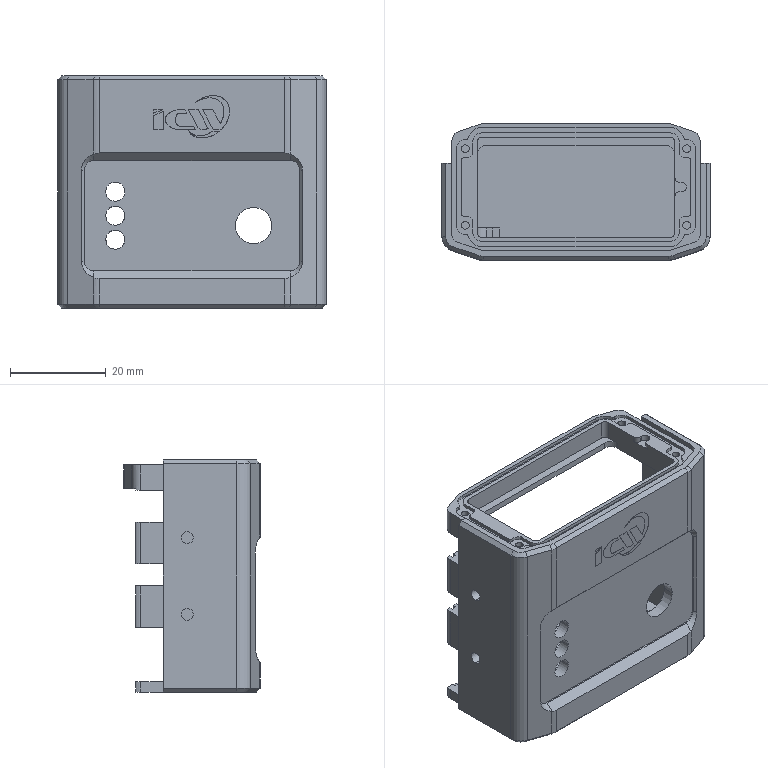Part | SolidWorks | features BaseBody 1 | 1 solid | 305 faces | box 56 x 28.5 x 48.5 mm | volume 15692 mm3 | plane 165 | cylinder 119 | cone 14 | spline 7 | commonest cylinder face diameters 4 x35 3.8 x18 1 x16 1.6 x8 2 x8 4.2 x8